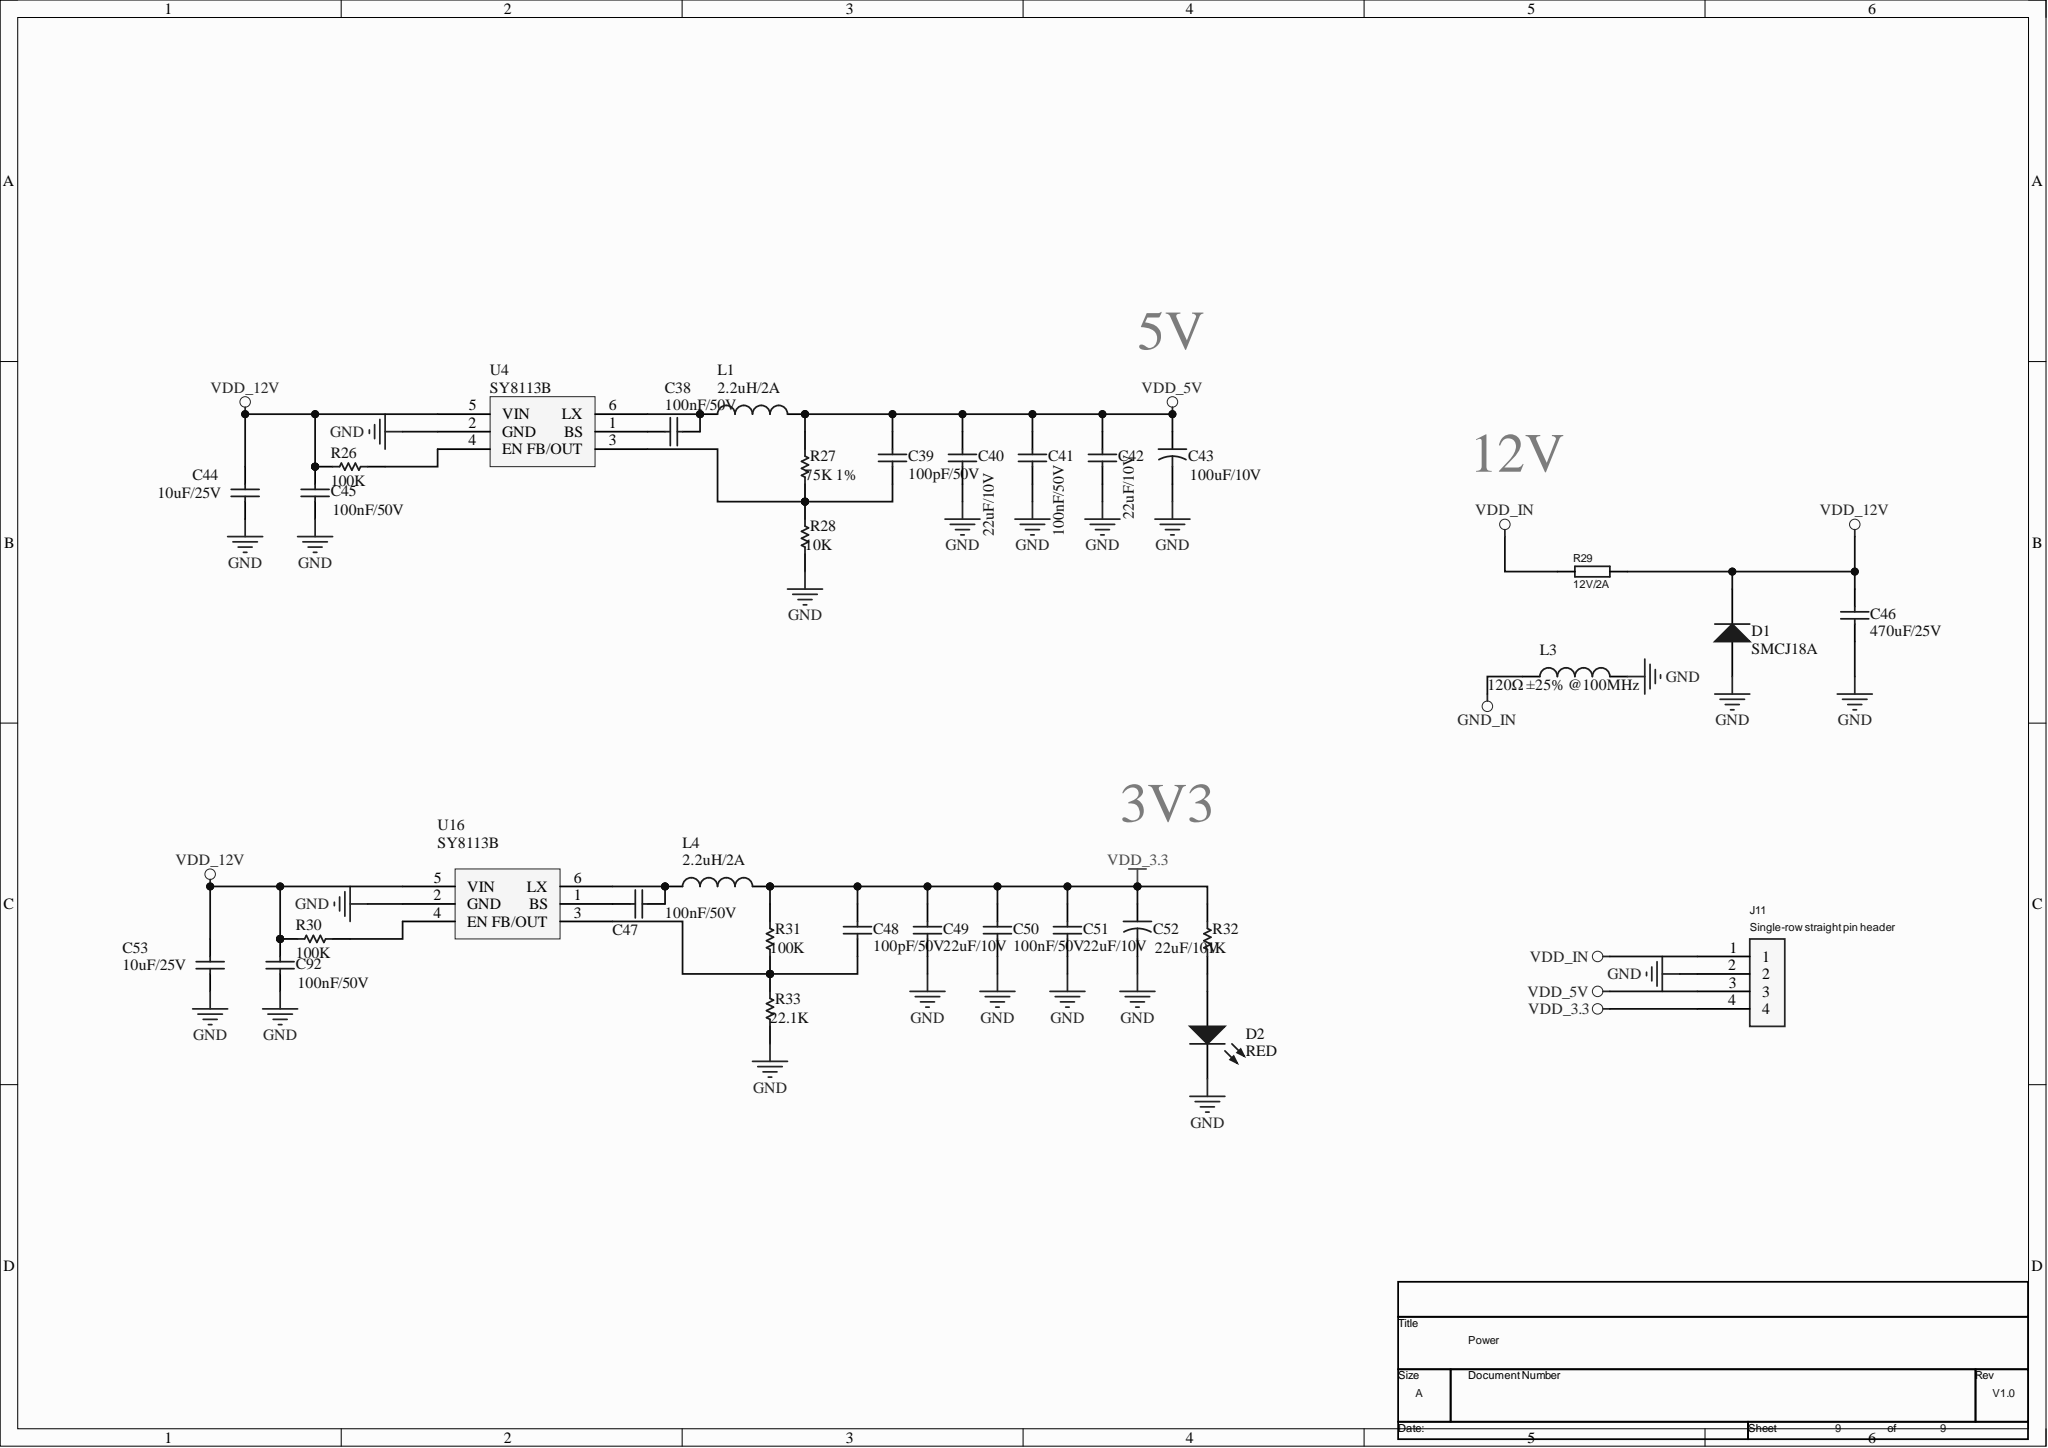Circuit board | Altium Designer | 313 parts | 216 nets | one sheet of the schematic
Parts on this sheet (reference | value | footprint):
C38 | 100nF/50V | 0603
C39 | 100pF/50V | 0603
C40 | 22uF/10V | C0805
C41 | 100nF/50V | 0603
C43 | 100uF/10V | CAP-TH_BD5.0-P2.00-D0.8-FD
C44 | 10uF/25V | C0805
C45 | 100nF/50V | 0603
C46 | 470uF/25V | CAP-TH_BD8.0-P3.50-D1.0-FD
C47 | 100nF/50V | 0603
C48 | 100pF/50V | 0603
C49 | 22uF/10V | C0805
C50 | 100nF/50V | 0603
C51 | 22uF/10V | C0805
C52 | 22uF/10V | C0805
C53 | 10uF/25V | C0805
C92 | 100nF/50V | 0603
D1 | SMCJ18A | SMC_L6.9-W5.9-LS7.9-RD
D2 | RED | LED_0805
J11 | Single-row straight pin header | HDR1X4
L1 | 2.2uH/2A | IND-SMD_L4.0-W4.0
L3 | 120Ω ±25% @100MHz | 0603
L4 | 2.2uH/2A | IND-SMD_L4.0-W4.0
R26 | 100K | 0603
R27 | 75K 1% | 0603
R28 | 10K | 0603
R29 | 12V/2A | 1210
R30 | 100K | 0603
R31 | 100K | 0603
R32 | 1K | 0603
R33 | 22.1K | 0603
U4 | SY8113B | TSOT-23-6_L2.9-W1.6-P0.95-LS2.8-BR
U16 | SY8113B | TSOT-23-6_L2.9-W1.6-P0.95-LS2.8-BR
Nets of these parts (net: part-pin ...):
VDD_IN: J11-1 R29-2
VDD_12V: C44-2 C45-2 C46-1 C53-2 C92-2 D1-2 R26-2 R29-1 R30-2 U4-5 U16-5
VDD_5V: C39-1 C40-1 C41-1 C43-1 J11-3 L1-2 R27-2
VDD_3.3: C48-1 C49-1 C50-1 C51-1 C52-1 J11-4 L4-2 R31-2 R32-2
NetR30_1: R30-1 U16-4
NetR26_1: R26-1 U4-4
NetD2_1: D2-1 R32-1
NetC48_2: C48-2 R31-1 R33-2 U16-3
NetC47_2: C47-2 U16-1
NetC47_1: C47-1 L4-1 U16-6
NetC39_2: C39-2 R27-1 R28-2 U4-3
NetC38_2: C38-2 U4-1
NetC38_1: C38-1 L1-1 U4-6
GND_IN: L3-1
GND: C40-2 C41-2 C43-2 C44-1 C45-1 C46-2 C49-2 C50-2 C51-2 C52-2 C53-1 C92-1 D1-1 D2-2 J11-2 L3-2 R28-1 R33-1 U4-2 U16-2